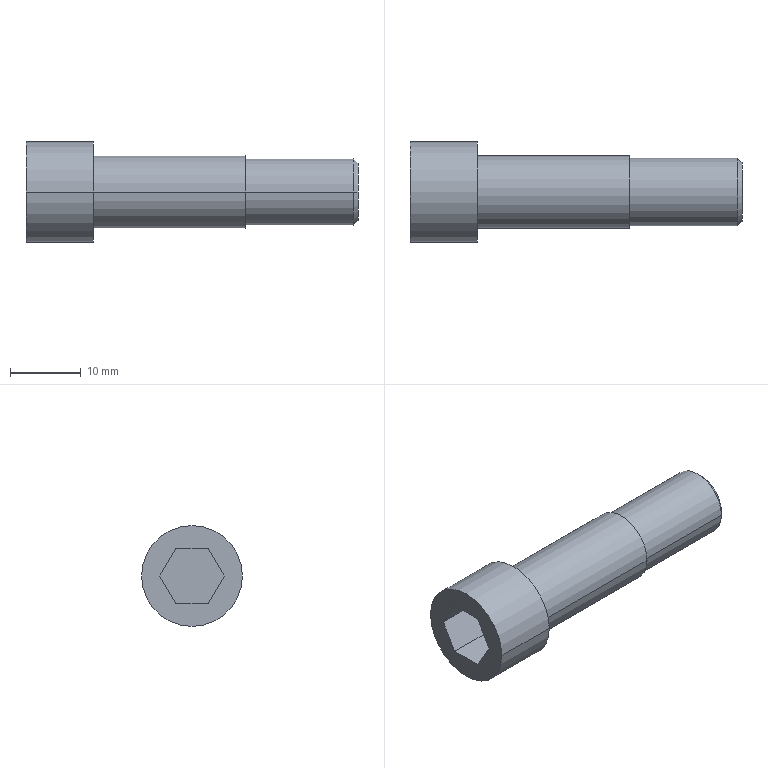Part | STEP file | 4-20.sldasm-Part-59 | 1 solid | 19 faces | box 47.085 x 14.288 x 14.288 mm | volume 4121 mm3 | plane 11 | cylinder 6 | cone 2 | commonest cylinder face diameters 9.525 x2 10.317 x2 14.288 x2
STEP:
#1=CARTESIAN_POINT('',(-241.51,381.926,175.9));
#2=VERTEX_POINT('',#1);
#3=CARTESIAN_POINT('',(-241.51,396.214,175.9));
#4=VERTEX_POINT('',#3);
#5=CARTESIAN_POINT('',(-241.51,389.07,175.9));
#6=DIRECTION('',(-1.,0.,0.));
#7=DIRECTION('',(0.,0.,1.));
#8=AXIS2_PLACEMENT_3D('',#5,#6,#7);
#9=CIRCLE('',#8,7.144);
#10=EDGE_CURVE('',#2,#4,#9,.T.);
#11=ORIENTED_EDGE('',*,*,#10,.T.);
#12=CARTESIAN_POINT('',(-251.035,396.214,175.9));
#13=VERTEX_POINT('',#12);
#14=CARTESIAN_POINT('',(-244.05,396.214,175.9));
#15=DIRECTION('',(-1.,0.,0.));
#16=VECTOR('',#15,1000.);
#17=LINE('',#14,#16);
#18=EDGE_CURVE('',#4,#13,#17,.T.);
#19=ORIENTED_EDGE('',*,*,#18,.T.);
#20=CARTESIAN_POINT('',(-251.035,381.926,175.9));
#21=VERTEX_POINT('',#20);
#22=CARTESIAN_POINT('',(-251.035,389.07,175.9));
#23=DIRECTION('',(-1.,0.,0.));
#24=DIRECTION('',(0.,0.,-1.));
#25=AXIS2_PLACEMENT_3D('',#22,#23,#24);
#26=CIRCLE('',#25,7.144);
#27=EDGE_CURVE('',#21,#13,#26,.T.);
#28=ORIENTED_EDGE('',*,*,#27,.F.);
#29=CARTESIAN_POINT('',(-244.05,381.926,175.9));
#30=DIRECTION('',(-1.,0.,0.));
#31=VECTOR('',#30,1000.);
#32=LINE('',#29,#31);
#33=EDGE_CURVE('',#2,#21,#32,.T.);
#34=ORIENTED_EDGE('',*,*,#33,.F.);
#35=EDGE_LOOP('',(#11,#19,#28,#34));
#36=FACE_OUTER_BOUND('',#35,.T.);
#37=CARTESIAN_POINT('',(-244.05,389.07,175.9));
#38=DIRECTION('',(-1.,0.,0.));
#39=DIRECTION('',(0.,-1.,0.));
#40=AXIS2_PLACEMENT_3D('',#37,#38,#39);
#41=CYLINDRICAL_SURFACE('',#40,7.144);
#42=ADVANCED_FACE('',(#36),#41,.T.);
#43=CARTESIAN_POINT('',(-241.51,383.911,175.9));
#44=VERTEX_POINT('',#43);
#45=CARTESIAN_POINT('',(-241.51,394.229,175.9));
#46=VERTEX_POINT('',#45);
#47=CARTESIAN_POINT('',(-241.51,389.07,175.9));
#48=DIRECTION('',(-1.,0.,0.));
#49=DIRECTION('',(0.,0.,1.));
#50=AXIS2_PLACEMENT_3D('',#47,#48,#49);
#51=CIRCLE('',#50,5.159);
#52=EDGE_CURVE('',#44,#46,#51,.T.);
#53=ORIENTED_EDGE('',*,*,#52,.F.);
#54=CARTESIAN_POINT('',(-219.92,383.911,175.9));
#55=VERTEX_POINT('',#54);
#56=CARTESIAN_POINT('',(-244.05,383.911,175.9));
#57=DIRECTION('',(1.,0.,0.));
#58=VECTOR('',#57,1000.);
#59=LINE('',#56,#58);
#60=EDGE_CURVE('',#44,#55,#59,.T.);
#61=ORIENTED_EDGE('',*,*,#60,.T.);
#62=CARTESIAN_POINT('',(-219.92,394.229,175.9));
#63=VERTEX_POINT('',#62);
#64=CARTESIAN_POINT('',(-219.92,389.07,175.9));
#65=DIRECTION('',(1.,0.,0.));
#66=DIRECTION('',(0.,0.,1.));
#67=AXIS2_PLACEMENT_3D('',#64,#65,#66);
#68=CIRCLE('',#67,5.159);
#69=EDGE_CURVE('',#63,#55,#68,.T.);
#70=ORIENTED_EDGE('',*,*,#69,.F.);
#71=CARTESIAN_POINT('',(-244.05,394.229,175.9));
#72=DIRECTION('',(1.,0.,0.));
#73=VECTOR('',#72,1000.);
#74=LINE('',#71,#73);
#75=EDGE_CURVE('',#46,#63,#74,.T.);
#76=ORIENTED_EDGE('',*,*,#75,.F.);
#77=EDGE_LOOP('',(#53,#61,#70,#76));
#78=FACE_OUTER_BOUND('',#77,.T.);
#79=CARTESIAN_POINT('',(-244.05,389.07,175.9));
#80=DIRECTION('',(1.,0.,0.));
#81=DIRECTION('',(0.,1.,0.));
#82=AXIS2_PLACEMENT_3D('',#79,#80,#81);
#83=CYLINDRICAL_SURFACE('',#82,5.159);
#84=ADVANCED_FACE('',(#78),#83,.T.);
#85=CARTESIAN_POINT('',(-219.92,393.833,175.9));
#86=VERTEX_POINT('',#85);
#87=CARTESIAN_POINT('',(-219.92,384.308,175.9));
#88=VERTEX_POINT('',#87);
#89=CARTESIAN_POINT('',(-219.92,389.07,175.9));
#90=DIRECTION('',(1.,0.,0.));
#91=DIRECTION('',(0.,0.,1.));
#92=AXIS2_PLACEMENT_3D('',#89,#90,#91);
#93=CIRCLE('',#92,4.763);
#94=EDGE_CURVE('',#86,#88,#93,.T.);
#95=ORIENTED_EDGE('',*,*,#94,.T.);
#96=CARTESIAN_POINT('',(-204.594,384.308,175.9));
#97=VERTEX_POINT('',#96);
#98=CARTESIAN_POINT('',(-244.05,384.308,175.9));
#99=DIRECTION('',(1.,0.,0.));
#100=VECTOR('',#99,1000.);
#101=LINE('',#98,#100);
#102=EDGE_CURVE('',#88,#97,#101,.T.);
#103=ORIENTED_EDGE('',*,*,#102,.T.);
#104=CARTESIAN_POINT('',(-204.594,393.833,175.9));
#105=VERTEX_POINT('',#104);
#106=CARTESIAN_POINT('',(-204.594,389.07,175.9));
#107=DIRECTION('',(-1.,0.,0.));
#108=DIRECTION('',(0.,-1.,0.));
#109=AXIS2_PLACEMENT_3D('',#106,#107,#108);
#110=CIRCLE('',#109,4.763);
#111=EDGE_CURVE('',#97,#105,#110,.T.);
#112=ORIENTED_EDGE('',*,*,#111,.T.);
#113=CARTESIAN_POINT('',(-244.05,393.833,175.9));
#114=DIRECTION('',(1.,0.,0.));
#115=VECTOR('',#114,1000.);
#116=LINE('',#113,#115);
#117=EDGE_CURVE('',#86,#105,#116,.T.);
#118=ORIENTED_EDGE('',*,*,#117,.F.);
#119=EDGE_LOOP('',(#95,#103,#112,#118));
#120=FACE_OUTER_BOUND('',#119,.T.);
#121=CARTESIAN_POINT('',(-244.05,389.07,175.9));
#122=DIRECTION('',(1.,0.,0.));
#123=DIRECTION('',(0.,1.,0.));
#124=AXIS2_PLACEMENT_3D('',#121,#122,#123);
#125=CYLINDRICAL_SURFACE('',#124,4.763);
#126=ADVANCED_FACE('',(#120),#125,.T.);
#127=CARTESIAN_POINT('',(-203.95,393.189,175.9));
#128=VERTEX_POINT('',#127);
#129=CARTESIAN_POINT('',(-203.95,384.951,175.9));
#130=VERTEX_POINT('',#129);
#131=CARTESIAN_POINT('',(-203.95,389.07,175.9));
#132=DIRECTION('',(1.,0.,0.));
#133=DIRECTION('',(0.,-1.,0.));
#134=AXIS2_PLACEMENT_3D('',#131,#132,#133);
#135=CIRCLE('',#134,4.119);
#136=EDGE_CURVE('',#128,#130,#135,.T.);
#137=ORIENTED_EDGE('',*,*,#136,.F.);
#138=CARTESIAN_POINT('',(-204.594,393.833,175.9));
#139=DIRECTION('',(-0.7071,0.7071,0.));
#140=VECTOR('',#139,1000.);
#141=LINE('',#138,#140);
#142=EDGE_CURVE('',#128,#105,#141,.T.);
#143=ORIENTED_EDGE('',*,*,#142,.T.);
#144=ORIENTED_EDGE('',*,*,#111,.F.);
#145=CARTESIAN_POINT('',(-204.594,384.308,175.9));
#146=DIRECTION('',(-0.7071,-0.7071,0.));
#147=VECTOR('',#146,1000.);
#148=LINE('',#145,#147);
#149=EDGE_CURVE('',#130,#97,#148,.T.);
#150=ORIENTED_EDGE('',*,*,#149,.F.);
#151=EDGE_LOOP('',(#137,#143,#144,#150));
#152=FACE_OUTER_BOUND('',#151,.T.);
#153=CARTESIAN_POINT('',(-204.594,389.07,175.9));
#154=DIRECTION('',(-1.,0.,0.));
#155=DIRECTION('',(0.,-1.,0.));
#156=AXIS2_PLACEMENT_3D('',#153,#154,#155);
#157=CONICAL_SURFACE('',#156,4.763,0.7854);
#158=ADVANCED_FACE('',(#152),#157,.T.);
#159=CARTESIAN_POINT('',(-203.95,389.07,175.9));
#160=DIRECTION('',(1.,0.,0.));
#161=DIRECTION('',(0.,-1.,0.));
#162=AXIS2_PLACEMENT_3D('',#159,#160,#161);
#163=CIRCLE('',#162,4.119);
#164=EDGE_CURVE('',#130,#128,#163,.T.);
#165=ORIENTED_EDGE('',*,*,#164,.T.);
#166=ORIENTED_EDGE('',*,*,#136,.T.);
#167=EDGE_LOOP('',(#165,#166));
#168=FACE_OUTER_BOUND('',#167,.T.);
#169=CARTESIAN_POINT('',(-203.95,389.07,175.9));
#170=DIRECTION('',(-1.,0.,0.));
#171=DIRECTION('',(0.,-1.,0.));
#172=AXIS2_PLACEMENT_3D('',#169,#170,#171);
#173=PLANE('',#172);
#174=ADVANCED_FACE('',(#168),#173,.F.);
#175=ORIENTED_EDGE('',*,*,#142,.F.);
#176=ORIENTED_EDGE('',*,*,#164,.F.);
#177=ORIENTED_EDGE('',*,*,#149,.T.);
#178=CARTESIAN_POINT('',(-204.594,389.07,175.9));
#179=DIRECTION('',(-1.,0.,0.));
#180=DIRECTION('',(0.,-1.,0.));
#181=AXIS2_PLACEMENT_3D('',#178,#179,#180);
#182=CIRCLE('',#181,4.763);
#183=EDGE_CURVE('',#105,#97,#182,.T.);
#184=ORIENTED_EDGE('',*,*,#183,.F.);
#185=EDGE_LOOP('',(#175,#176,#177,#184));
#186=FACE_OUTER_BOUND('',#185,.T.);
#187=CARTESIAN_POINT('',(-204.594,389.07,175.9));
#188=DIRECTION('',(-1.,0.,0.));
#189=DIRECTION('',(0.,-1.,0.));
#190=AXIS2_PLACEMENT_3D('',#187,#188,#189);
#191=CONICAL_SURFACE('',#190,4.763,0.7854);
#192=ADVANCED_FACE('',(#186),#191,.T.);
#193=ORIENTED_EDGE('',*,*,#102,.F.);
#194=CARTESIAN_POINT('',(-219.92,389.07,175.9));
#195=DIRECTION('',(1.,0.,0.));
#196=DIRECTION('',(0.,0.,1.));
#197=AXIS2_PLACEMENT_3D('',#194,#195,#196);
#198=CIRCLE('',#197,4.763);
#199=EDGE_CURVE('',#88,#86,#198,.T.);
#200=ORIENTED_EDGE('',*,*,#199,.T.);
#201=ORIENTED_EDGE('',*,*,#117,.T.);
#202=ORIENTED_EDGE('',*,*,#183,.T.);
#203=EDGE_LOOP('',(#193,#200,#201,#202));
#204=FACE_OUTER_BOUND('',#203,.T.);
#205=CARTESIAN_POINT('',(-244.05,389.07,175.9));
#206=DIRECTION('',(1.,0.,0.));
#207=DIRECTION('',(0.,1.,0.));
#208=AXIS2_PLACEMENT_3D('',#205,#206,#207);
#209=CYLINDRICAL_SURFACE('',#208,4.763);
#210=ADVANCED_FACE('',(#204),#209,.T.);
#211=ORIENTED_EDGE('',*,*,#69,.T.);
#212=CARTESIAN_POINT('',(-219.92,389.07,175.9));
#213=DIRECTION('',(1.,0.,0.));
#214=DIRECTION('',(0.,0.,1.));
#215=AXIS2_PLACEMENT_3D('',#212,#213,#214);
#216=CIRCLE('',#215,5.159);
#217=EDGE_CURVE('',#55,#63,#216,.T.);
#218=ORIENTED_EDGE('',*,*,#217,.T.);
#219=EDGE_LOOP('',(#211,#218));
#220=FACE_OUTER_BOUND('',#219,.T.);
#221=ORIENTED_EDGE('',*,*,#94,.F.);
#222=ORIENTED_EDGE('',*,*,#199,.F.);
#223=EDGE_LOOP('',(#221,#222));
#224=FACE_BOUND('',#223,.T.);
#225=CARTESIAN_POINT('',(-219.92,389.07,150.5));
#226=DIRECTION('',(1.,0.,0.));
#227=DIRECTION('',(0.,0.,1.));
#228=AXIS2_PLACEMENT_3D('',#225,#226,#227);
#229=PLANE('',#228);
#230=ADVANCED_FACE('',(#220,#224),#229,.T.);
#231=ORIENTED_EDGE('',*,*,#60,.F.);
#232=CARTESIAN_POINT('',(-241.51,389.07,175.9));
#233=DIRECTION('',(-1.,0.,0.));
#234=DIRECTION('',(0.,0.,1.));
#235=AXIS2_PLACEMENT_3D('',#232,#233,#234);
#236=CIRCLE('',#235,5.159);
#237=EDGE_CURVE('',#46,#44,#236,.T.);
#238=ORIENTED_EDGE('',*,*,#237,.F.);
#239=ORIENTED_EDGE('',*,*,#75,.T.);
#240=ORIENTED_EDGE('',*,*,#217,.F.);
#241=EDGE_LOOP('',(#231,#238,#239,#240));
#242=FACE_OUTER_BOUND('',#241,.T.);
#243=CARTESIAN_POINT('',(-244.05,389.07,175.9));
#244=DIRECTION('',(1.,0.,0.));
#245=DIRECTION('',(0.,1.,0.));
#246=AXIS2_PLACEMENT_3D('',#243,#244,#245);
#247=CYLINDRICAL_SURFACE('',#246,5.159);
#248=ADVANCED_FACE('',(#242),#247,.T.);
#249=ORIENTED_EDGE('',*,*,#10,.F.);
#250=CARTESIAN_POINT('',(-241.51,389.07,175.9));
#251=DIRECTION('',(-1.,0.,0.));
#252=DIRECTION('',(0.,0.,1.));
#253=AXIS2_PLACEMENT_3D('',#250,#251,#252);
#254=CIRCLE('',#253,7.144);
#255=EDGE_CURVE('',#4,#2,#254,.T.);
#256=ORIENTED_EDGE('',*,*,#255,.F.);
#257=EDGE_LOOP('',(#249,#256));
#258=FACE_OUTER_BOUND('',#257,.T.);
#259=ORIENTED_EDGE('',*,*,#237,.T.);
#260=ORIENTED_EDGE('',*,*,#52,.T.);
#261=EDGE_LOOP('',(#259,#260));
#262=FACE_BOUND('',#261,.T.);
#263=CARTESIAN_POINT('',(-241.51,389.07,175.9));
#264=DIRECTION('',(1.,0.,0.));
#265=DIRECTION('',(0.,1.,0.));
#266=AXIS2_PLACEMENT_3D('',#263,#264,#265);
#267=PLANE('',#266);
#268=ADVANCED_FACE('',(#258,#262),#267,.T.);
#269=CARTESIAN_POINT('',(-251.035,391.361,171.931));
#270=VERTEX_POINT('',#269);
#271=CARTESIAN_POINT('',(-251.035,386.779,171.931));
#272=VERTEX_POINT('',#271);
#273=CARTESIAN_POINT('',(-251.035,389.07,171.931));
#274=DIRECTION('',(0.,-1.,0.));
#275=VECTOR('',#274,1000.);
#276=LINE('',#273,#275);
#277=EDGE_CURVE('',#270,#272,#276,.T.);
#278=ORIENTED_EDGE('',*,*,#277,.F.);
#279=CARTESIAN_POINT('',(-251.035,393.653,175.9));
#280=VERTEX_POINT('',#279);
#281=CARTESIAN_POINT('',(-251.035,392.507,173.916));
#282=DIRECTION('',(0.,-0.5,-0.866));
#283=VECTOR('',#282,1000.);
#284=LINE('',#281,#283);
#285=EDGE_CURVE('',#280,#270,#284,.T.);
#286=ORIENTED_EDGE('',*,*,#285,.F.);
#287=CARTESIAN_POINT('',(-251.035,391.361,179.869));
#288=VERTEX_POINT('',#287);
#289=CARTESIAN_POINT('',(-251.035,392.507,177.884));
#290=DIRECTION('',(0.,0.5,-0.866));
#291=VECTOR('',#290,1000.);
#292=LINE('',#289,#291);
#293=EDGE_CURVE('',#288,#280,#292,.T.);
#294=ORIENTED_EDGE('',*,*,#293,.F.);
#295=CARTESIAN_POINT('',(-251.035,386.779,179.869));
#296=VERTEX_POINT('',#295);
#297=CARTESIAN_POINT('',(-251.035,389.07,179.869));
#298=DIRECTION('',(0.,1.,0.));
#299=VECTOR('',#298,1000.);
#300=LINE('',#297,#299);
#301=EDGE_CURVE('',#296,#288,#300,.T.);
#302=ORIENTED_EDGE('',*,*,#301,.F.);
#303=CARTESIAN_POINT('',(-251.035,384.487,175.9));
#304=VERTEX_POINT('',#303);
#305=CARTESIAN_POINT('',(-251.035,385.633,177.884));
#306=DIRECTION('',(0.,0.5,0.866));
#307=VECTOR('',#306,1000.);
#308=LINE('',#305,#307);
#309=EDGE_CURVE('',#304,#296,#308,.T.);
#310=ORIENTED_EDGE('',*,*,#309,.F.);
#311=CARTESIAN_POINT('',(-251.035,385.633,173.916));
#312=DIRECTION('',(0.,-0.5,0.866));
#313=VECTOR('',#312,1000.);
#314=LINE('',#311,#313);
#315=EDGE_CURVE('',#272,#304,#314,.T.);
#316=ORIENTED_EDGE('',*,*,#315,.F.);
#317=EDGE_LOOP('',(#278,#286,#294,#302,#310,#316));
#318=FACE_BOUND('',#317,.T.);
#319=ORIENTED_EDGE('',*,*,#27,.T.);
#320=CARTESIAN_POINT('',(-251.035,389.07,175.9));
#321=DIRECTION('',(-1.,0.,0.));
#322=DIRECTION('',(0.,0.,-1.));
#323=AXIS2_PLACEMENT_3D('',#320,#321,#322);
#324=CIRCLE('',#323,7.144);
#325=EDGE_CURVE('',#13,#21,#324,.T.);
#326=ORIENTED_EDGE('',*,*,#325,.T.);
#327=EDGE_LOOP('',(#319,#326));
#328=FACE_OUTER_BOUND('',#327,.T.);
#329=CARTESIAN_POINT('',(-251.035,389.07,175.9));
#330=DIRECTION('',(-1.,0.,0.));
#331=DIRECTION('',(0.,-1.,0.));
#332=AXIS2_PLACEMENT_3D('',#329,#330,#331);
#333=PLANE('',#332);
#334=ADVANCED_FACE('',(#318,#328),#333,.T.);
#335=ORIENTED_EDGE('',*,*,#18,.F.);
#336=ORIENTED_EDGE('',*,*,#255,.T.);
#337=ORIENTED_EDGE('',*,*,#33,.T.);
#338=ORIENTED_EDGE('',*,*,#325,.F.);
#339=EDGE_LOOP('',(#335,#336,#337,#338));
#340=FACE_OUTER_BOUND('',#339,.T.);
#341=CARTESIAN_POINT('',(-244.05,389.07,175.9));
#342=DIRECTION('',(-1.,0.,0.));
#343=DIRECTION('',(0.,-1.,0.));
#344=AXIS2_PLACEMENT_3D('',#341,#342,#343);
#345=CYLINDRICAL_SURFACE('',#344,7.144);
#346=ADVANCED_FACE('',(#340),#345,.T.);
#347=ORIENTED_EDGE('',*,*,#277,.T.);
#348=CARTESIAN_POINT('',(-244.748,386.779,171.931));
#349=VERTEX_POINT('',#348);
#350=CARTESIAN_POINT('',(-247.288,386.779,171.931));
#351=DIRECTION('',(-1.,0.,0.));
#352=VECTOR('',#351,1000.);
#353=LINE('',#350,#352);
#354=EDGE_CURVE('',#349,#272,#353,.T.);
#355=ORIENTED_EDGE('',*,*,#354,.F.);
#356=CARTESIAN_POINT('',(-244.748,391.361,171.931));
#357=VERTEX_POINT('',#356);
#358=CARTESIAN_POINT('',(-244.748,386.779,171.931));
#359=DIRECTION('',(0.,-1.,0.));
#360=VECTOR('',#359,1000.);
#361=LINE('',#358,#360);
#362=EDGE_CURVE('',#357,#349,#361,.T.);
#363=ORIENTED_EDGE('',*,*,#362,.F.);
#364=CARTESIAN_POINT('',(-247.288,391.361,171.931));
#365=DIRECTION('',(-1.,0.,0.));
#366=VECTOR('',#365,1000.);
#367=LINE('',#364,#366);
#368=EDGE_CURVE('',#357,#270,#367,.T.);
#369=ORIENTED_EDGE('',*,*,#368,.T.);
#370=EDGE_LOOP('',(#347,#355,#363,#369));
#371=FACE_OUTER_BOUND('',#370,.T.);
#372=CARTESIAN_POINT('',(-247.288,391.361,171.931));
#373=DIRECTION('',(0.,0.,-1.));
#374=DIRECTION('',(1.,0.,0.));
#375=AXIS2_PLACEMENT_3D('',#372,#373,#374);
#376=PLANE('',#375);
#377=ADVANCED_FACE('',(#371),#376,.F.);
#378=ORIENTED_EDGE('',*,*,#315,.T.);
#379=CARTESIAN_POINT('',(-244.748,384.487,175.9));
#380=VERTEX_POINT('',#379);
#381=CARTESIAN_POINT('',(-247.288,384.487,175.9));
#382=DIRECTION('',(-1.,0.,0.));
#383=VECTOR('',#382,1000.);
#384=LINE('',#381,#383);
#385=EDGE_CURVE('',#380,#304,#384,.T.);
#386=ORIENTED_EDGE('',*,*,#385,.F.);
#387=CARTESIAN_POINT('',(-244.748,386.779,171.931));
#388=DIRECTION('',(0.,-0.5,0.866));
#389=VECTOR('',#388,1000.);
#390=LINE('',#387,#389);
#391=EDGE_CURVE('',#349,#380,#390,.T.);
#392=ORIENTED_EDGE('',*,*,#391,.F.);
#393=ORIENTED_EDGE('',*,*,#354,.T.);
#394=EDGE_LOOP('',(#378,#386,#392,#393));
#395=FACE_OUTER_BOUND('',#394,.T.);
#396=CARTESIAN_POINT('',(-247.288,386.779,171.931));
#397=DIRECTION('',(0.,-0.866,-0.5));
#398=DIRECTION('',(0.,-0.5,0.866));
#399=AXIS2_PLACEMENT_3D('',#396,#397,#398);
#400=PLANE('',#399);
#401=ADVANCED_FACE('',(#395),#400,.F.);
#402=ORIENTED_EDGE('',*,*,#309,.T.);
#403=CARTESIAN_POINT('',(-244.748,386.779,179.869));
#404=VERTEX_POINT('',#403);
#405=CARTESIAN_POINT('',(-247.288,386.779,179.869));
#406=DIRECTION('',(-1.,0.,0.));
#407=VECTOR('',#406,1000.);
#408=LINE('',#405,#407);
#409=EDGE_CURVE('',#404,#296,#408,.T.);
#410=ORIENTED_EDGE('',*,*,#409,.F.);
#411=CARTESIAN_POINT('',(-244.748,383.342,173.916));
#412=DIRECTION('',(0.,0.5,0.866));
#413=VECTOR('',#412,1000.);
#414=LINE('',#411,#413);
#415=EDGE_CURVE('',#380,#404,#414,.T.);
#416=ORIENTED_EDGE('',*,*,#415,.F.);
#417=ORIENTED_EDGE('',*,*,#385,.T.);
#418=EDGE_LOOP('',(#402,#410,#416,#417));
#419=FACE_OUTER_BOUND('',#418,.T.);
#420=CARTESIAN_POINT('',(-247.288,384.487,175.9));
#421=DIRECTION('',(0.,-0.866,0.5));
#422=DIRECTION('',(0.,0.5,0.866));
#423=AXIS2_PLACEMENT_3D('',#420,#421,#422);
#424=PLANE('',#423);
#425=ADVANCED_FACE('',(#419),#424,.F.);
#426=ORIENTED_EDGE('',*,*,#301,.T.);
#427=CARTESIAN_POINT('',(-244.748,391.361,179.869));
#428=VERTEX_POINT('',#427);
#429=CARTESIAN_POINT('',(-247.288,391.361,179.869));
#430=DIRECTION('',(-1.,0.,0.));
#431=VECTOR('',#430,1000.);
#432=LINE('',#429,#431);
#433=EDGE_CURVE('',#428,#288,#432,.T.);
#434=ORIENTED_EDGE('',*,*,#433,.F.);
#435=CARTESIAN_POINT('',(-244.748,386.779,179.869));
#436=DIRECTION('',(0.,1.,0.));
#437=VECTOR('',#436,1000.);
#438=LINE('',#435,#437);
#439=EDGE_CURVE('',#404,#428,#438,.T.);
#440=ORIENTED_EDGE('',*,*,#439,.F.);
#441=ORIENTED_EDGE('',*,*,#409,.T.);
#442=EDGE_LOOP('',(#426,#434,#440,#441));
#443=FACE_OUTER_BOUND('',#442,.T.);
#444=CARTESIAN_POINT('',(-247.288,386.779,179.869));
#445=DIRECTION('',(0.,0.,1.));
#446=DIRECTION('',(-1.,0.,0.));
#447=AXIS2_PLACEMENT_3D('',#444,#445,#446);
#448=PLANE('',#447);
#449=ADVANCED_FACE('',(#443),#448,.F.);
#450=ORIENTED_EDGE('',*,*,#293,.T.);
#451=CARTESIAN_POINT('',(-244.748,393.653,175.9));
#452=VERTEX_POINT('',#451);
#453=CARTESIAN_POINT('',(-247.288,393.653,175.9));
#454=DIRECTION('',(-1.,0.,0.));
#455=VECTOR('',#454,1000.);
#456=LINE('',#453,#455);
#457=EDGE_CURVE('',#452,#280,#456,.T.);
#458=ORIENTED_EDGE('',*,*,#457,.F.);
#459=CARTESIAN_POINT('',(-244.748,393.653,175.9));
#460=DIRECTION('',(0.,0.5,-0.866));
#461=VECTOR('',#460,1000.);
#462=LINE('',#459,#461);
#463=EDGE_CURVE('',#428,#452,#462,.T.);
#464=ORIENTED_EDGE('',*,*,#463,.F.);
#465=ORIENTED_EDGE('',*,*,#433,.T.);
#466=EDGE_LOOP('',(#450,#458,#464,#465));
#467=FACE_OUTER_BOUND('',#466,.T.);
#468=CARTESIAN_POINT('',(-247.288,391.361,179.869));
#469=DIRECTION('',(0.,0.866,0.5));
#470=DIRECTION('',(0.,0.5,-0.866));
#471=AXIS2_PLACEMENT_3D('',#468,#469,#470);
#472=PLANE('',#471);
#473=ADVANCED_FACE('',(#467),#472,.F.);
#474=ORIENTED_EDGE('',*,*,#285,.T.);
#475=ORIENTED_EDGE('',*,*,#368,.F.);
#476=CARTESIAN_POINT('',(-244.748,390.216,169.947));
#477=DIRECTION('',(0.,-0.5,-0.866));
#478=VECTOR('',#477,1000.);
#479=LINE('',#476,#478);
#480=EDGE_CURVE('',#452,#357,#479,.T.);
#481=ORIENTED_EDGE('',*,*,#480,.F.);
#482=ORIENTED_EDGE('',*,*,#457,.T.);
#483=EDGE_LOOP('',(#474,#475,#481,#482));
#484=FACE_OUTER_BOUND('',#483,.T.);
#485=CARTESIAN_POINT('',(-247.288,393.653,175.9));
#486=DIRECTION('',(0.,0.866,-0.5));
#487=DIRECTION('',(0.,-0.5,-0.866));
#488=AXIS2_PLACEMENT_3D('',#485,#486,#487);
#489=PLANE('',#488);
#490=ADVANCED_FACE('',(#484),#489,.F.);
#491=ORIENTED_EDGE('',*,*,#362,.T.);
#492=ORIENTED_EDGE('',*,*,#391,.T.);
#493=ORIENTED_EDGE('',*,*,#415,.T.);
#494=ORIENTED_EDGE('',*,*,#439,.T.);
#495=ORIENTED_EDGE('',*,*,#463,.T.);
#496=ORIENTED_EDGE('',*,*,#480,.T.);
#497=EDGE_LOOP('',(#491,#492,#493,#494,#495,#496));
#498=FACE_OUTER_BOUND('',#497,.T.);
#499=CARTESIAN_POINT('',(-244.748,386.779,171.931));
#500=DIRECTION('',(-1.,0.,0.));
#501=DIRECTION('',(0.,-1.,0.));
#502=AXIS2_PLACEMENT_3D('',#499,#500,#501);
#503=PLANE('',#502);
#504=ADVANCED_FACE('',(#498),#503,.T.);
#505=CLOSED_SHELL('',(#42,#84,#126,#158,#174,#192,#210,#230,#248,#268,#334,#346,#377,#401,#425,#449,#473,#490,#504));
#506=MANIFOLD_SOLID_BREP('',#505);
#507=CARTESIAN_POINT('',(0.,0.,0.));
#508=DIRECTION('',(0.,0.,1.));
#509=DIRECTION('',(1.,0.,0.));
#510=AXIS2_PLACEMENT_3D('',#507,#508,#509);
#511=(LENGTH_UNIT()NAMED_UNIT(*)SI_UNIT(.MILLI.,.METRE.));
#512=UNCERTAINTY_MEASURE_WITH_UNIT(LENGTH_MEASURE(0.00001),#511,'','');
#513=(NAMED_UNIT(*)PLANE_ANGLE_UNIT()SI_UNIT($,.RADIAN.));
#514=(NAMED_UNIT(*)SI_UNIT($,.STERADIAN.)SOLID_ANGLE_UNIT());
#515=(GEOMETRIC_REPRESENTATION_CONTEXT(3)GLOBAL_UNCERTAINTY_ASSIGNED_CONTEXT((#512))GLOBAL_UNIT_ASSIGNED_CONTEXT((#511,#513,#514))REPRESENTATION_CONTEXT('',''));
#516=ADVANCED_BREP_SHAPE_REPRESENTATION('',(#506,#510),#515);